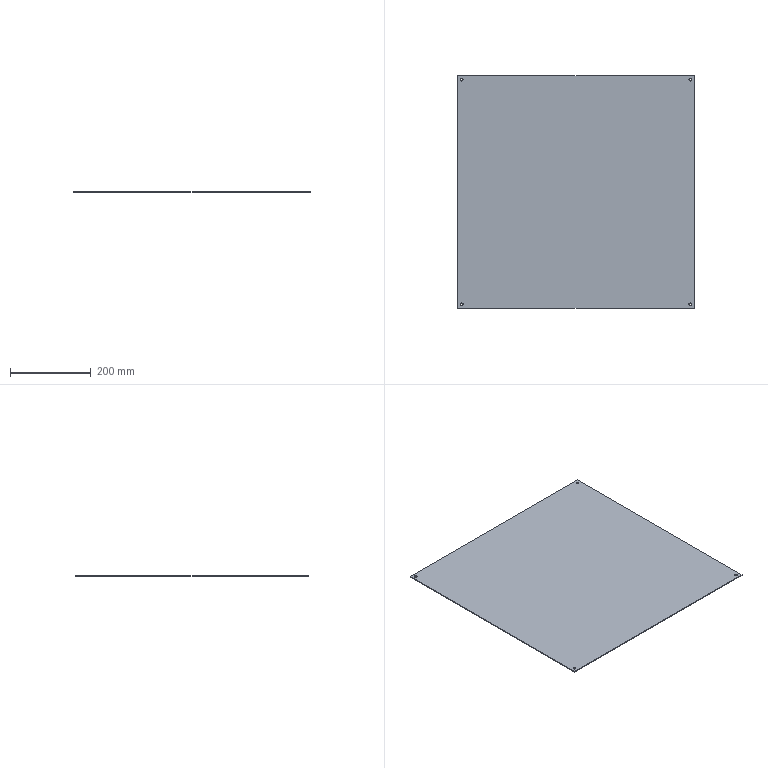Part | SolidWorks | features FlatPattern 1, HoleWzd 1, SMBaseFlange 1, SheetMetal 1 | 1 solid | 14 faces | box 587 x 577 x 2 mm | volume 677090 mm3 | cylinder 8 | plane 6 | commonest cylinder face diameters 7 x8
STEP:
#1=CARTESIAN_POINT('',(-287.,278.5,-2.));
#2=VERTEX_POINT('',#1);
#3=CARTESIAN_POINT('',(-280.,278.5,-2.));
#4=VERTEX_POINT('',#3);
#5=CARTESIAN_POINT('',(-283.5,278.5,-2.));
#6=DIRECTION('',(0.,0.,1.));
#7=DIRECTION('',(1.,0.,0.));
#8=AXIS2_PLACEMENT_3D('',#5,#6,#7);
#9=CIRCLE('',#8,3.5);
#10=EDGE_CURVE('',#2,#4,#9,.T.);
#11=ORIENTED_EDGE('',*,*,#10,.F.);
#12=CARTESIAN_POINT('',(-287.,278.5,0.));
#13=VERTEX_POINT('',#12);
#14=CARTESIAN_POINT('',(-287.,278.5,0.));
#15=DIRECTION('',(0.,0.,1.));
#16=VECTOR('',#15,1000.);
#17=LINE('',#14,#16);
#18=EDGE_CURVE('',#2,#13,#17,.T.);
#19=ORIENTED_EDGE('',*,*,#18,.T.);
#20=CARTESIAN_POINT('',(-280.,278.5,0.));
#21=VERTEX_POINT('',#20);
#22=CARTESIAN_POINT('',(-283.5,278.5,0.));
#23=DIRECTION('',(0.,0.,1.));
#24=DIRECTION('',(1.,0.,0.));
#25=AXIS2_PLACEMENT_3D('',#22,#23,#24);
#26=CIRCLE('',#25,3.5);
#27=EDGE_CURVE('',#13,#21,#26,.T.);
#28=ORIENTED_EDGE('',*,*,#27,.T.);
#29=CARTESIAN_POINT('',(-280.,278.5,0.));
#30=DIRECTION('',(0.,0.,1.));
#31=VECTOR('',#30,1000.);
#32=LINE('',#29,#31);
#33=EDGE_CURVE('',#4,#21,#32,.T.);
#34=ORIENTED_EDGE('',*,*,#33,.F.);
#35=EDGE_LOOP('',(#11,#19,#28,#34));
#36=FACE_OUTER_BOUND('',#35,.T.);
#37=CARTESIAN_POINT('',(-283.5,278.5,0.));
#38=DIRECTION('',(0.,0.,1.));
#39=DIRECTION('',(1.,0.,0.));
#40=AXIS2_PLACEMENT_3D('',#37,#38,#39);
#41=CYLINDRICAL_SURFACE('',#40,3.5);
#42=ADVANCED_FACE('',(#36),#41,.F.);
#43=CARTESIAN_POINT('',(-287.,-278.5,-2.));
#44=VERTEX_POINT('',#43);
#45=CARTESIAN_POINT('',(-280.,-278.5,-2.));
#46=VERTEX_POINT('',#45);
#47=CARTESIAN_POINT('',(-283.5,-278.5,-2.));
#48=DIRECTION('',(0.,0.,1.));
#49=DIRECTION('',(1.,0.,0.));
#50=AXIS2_PLACEMENT_3D('',#47,#48,#49);
#51=CIRCLE('',#50,3.5);
#52=EDGE_CURVE('',#44,#46,#51,.T.);
#53=ORIENTED_EDGE('',*,*,#52,.F.);
#54=CARTESIAN_POINT('',(-287.,-278.5,0.));
#55=VERTEX_POINT('',#54);
#56=CARTESIAN_POINT('',(-287.,-278.5,0.));
#57=DIRECTION('',(0.,0.,1.));
#58=VECTOR('',#57,1000.);
#59=LINE('',#56,#58);
#60=EDGE_CURVE('',#44,#55,#59,.T.);
#61=ORIENTED_EDGE('',*,*,#60,.T.);
#62=CARTESIAN_POINT('',(-280.,-278.5,0.));
#63=VERTEX_POINT('',#62);
#64=CARTESIAN_POINT('',(-283.5,-278.5,0.));
#65=DIRECTION('',(0.,0.,1.));
#66=DIRECTION('',(1.,0.,0.));
#67=AXIS2_PLACEMENT_3D('',#64,#65,#66);
#68=CIRCLE('',#67,3.5);
#69=EDGE_CURVE('',#55,#63,#68,.T.);
#70=ORIENTED_EDGE('',*,*,#69,.T.);
#71=CARTESIAN_POINT('',(-280.,-278.5,0.));
#72=DIRECTION('',(0.,0.,1.));
#73=VECTOR('',#72,1000.);
#74=LINE('',#71,#73);
#75=EDGE_CURVE('',#46,#63,#74,.T.);
#76=ORIENTED_EDGE('',*,*,#75,.F.);
#77=EDGE_LOOP('',(#53,#61,#70,#76));
#78=FACE_OUTER_BOUND('',#77,.T.);
#79=CARTESIAN_POINT('',(-283.5,-278.5,0.));
#80=DIRECTION('',(0.,0.,1.));
#81=DIRECTION('',(1.,0.,0.));
#82=AXIS2_PLACEMENT_3D('',#79,#80,#81);
#83=CYLINDRICAL_SURFACE('',#82,3.5);
#84=ADVANCED_FACE('',(#78),#83,.F.);
#85=CARTESIAN_POINT('',(280.,-278.5,-2.));
#86=VERTEX_POINT('',#85);
#87=CARTESIAN_POINT('',(287.,-278.5,-2.));
#88=VERTEX_POINT('',#87);
#89=CARTESIAN_POINT('',(283.5,-278.5,-2.));
#90=DIRECTION('',(0.,0.,1.));
#91=DIRECTION('',(1.,0.,0.));
#92=AXIS2_PLACEMENT_3D('',#89,#90,#91);
#93=CIRCLE('',#92,3.5);
#94=EDGE_CURVE('',#86,#88,#93,.T.);
#95=ORIENTED_EDGE('',*,*,#94,.F.);
#96=CARTESIAN_POINT('',(280.,-278.5,0.));
#97=VERTEX_POINT('',#96);
#98=CARTESIAN_POINT('',(280.,-278.5,0.));
#99=DIRECTION('',(0.,0.,1.));
#100=VECTOR('',#99,1000.);
#101=LINE('',#98,#100);
#102=EDGE_CURVE('',#86,#97,#101,.T.);
#103=ORIENTED_EDGE('',*,*,#102,.T.);
#104=CARTESIAN_POINT('',(287.,-278.5,0.));
#105=VERTEX_POINT('',#104);
#106=CARTESIAN_POINT('',(283.5,-278.5,0.));
#107=DIRECTION('',(0.,0.,1.));
#108=DIRECTION('',(1.,0.,0.));
#109=AXIS2_PLACEMENT_3D('',#106,#107,#108);
#110=CIRCLE('',#109,3.5);
#111=EDGE_CURVE('',#97,#105,#110,.T.);
#112=ORIENTED_EDGE('',*,*,#111,.T.);
#113=CARTESIAN_POINT('',(287.,-278.5,0.));
#114=DIRECTION('',(0.,0.,1.));
#115=VECTOR('',#114,1000.);
#116=LINE('',#113,#115);
#117=EDGE_CURVE('',#88,#105,#116,.T.);
#118=ORIENTED_EDGE('',*,*,#117,.F.);
#119=EDGE_LOOP('',(#95,#103,#112,#118));
#120=FACE_OUTER_BOUND('',#119,.T.);
#121=CARTESIAN_POINT('',(283.5,-278.5,0.));
#122=DIRECTION('',(0.,0.,1.));
#123=DIRECTION('',(1.,0.,0.));
#124=AXIS2_PLACEMENT_3D('',#121,#122,#123);
#125=CYLINDRICAL_SURFACE('',#124,3.5);
#126=ADVANCED_FACE('',(#120),#125,.F.);
#127=CARTESIAN_POINT('',(280.,278.5,-2.));
#128=VERTEX_POINT('',#127);
#129=CARTESIAN_POINT('',(287.,278.5,-2.));
#130=VERTEX_POINT('',#129);
#131=CARTESIAN_POINT('',(283.5,278.5,-2.));
#132=DIRECTION('',(0.,0.,1.));
#133=DIRECTION('',(1.,0.,0.));
#134=AXIS2_PLACEMENT_3D('',#131,#132,#133);
#135=CIRCLE('',#134,3.5);
#136=EDGE_CURVE('',#128,#130,#135,.T.);
#137=ORIENTED_EDGE('',*,*,#136,.F.);
#138=CARTESIAN_POINT('',(280.,278.5,0.));
#139=VERTEX_POINT('',#138);
#140=CARTESIAN_POINT('',(280.,278.5,0.));
#141=DIRECTION('',(0.,0.,1.));
#142=VECTOR('',#141,1000.);
#143=LINE('',#140,#142);
#144=EDGE_CURVE('',#128,#139,#143,.T.);
#145=ORIENTED_EDGE('',*,*,#144,.T.);
#146=CARTESIAN_POINT('',(287.,278.5,0.));
#147=VERTEX_POINT('',#146);
#148=CARTESIAN_POINT('',(283.5,278.5,0.));
#149=DIRECTION('',(0.,0.,1.));
#150=DIRECTION('',(1.,0.,0.));
#151=AXIS2_PLACEMENT_3D('',#148,#149,#150);
#152=CIRCLE('',#151,3.5);
#153=EDGE_CURVE('',#139,#147,#152,.T.);
#154=ORIENTED_EDGE('',*,*,#153,.T.);
#155=CARTESIAN_POINT('',(287.,278.5,0.));
#156=DIRECTION('',(0.,0.,1.));
#157=VECTOR('',#156,1000.);
#158=LINE('',#155,#157);
#159=EDGE_CURVE('',#130,#147,#158,.T.);
#160=ORIENTED_EDGE('',*,*,#159,.F.);
#161=EDGE_LOOP('',(#137,#145,#154,#160));
#162=FACE_OUTER_BOUND('',#161,.T.);
#163=CARTESIAN_POINT('',(283.5,278.5,0.));
#164=DIRECTION('',(0.,0.,1.));
#165=DIRECTION('',(1.,0.,0.));
#166=AXIS2_PLACEMENT_3D('',#163,#164,#165);
#167=CYLINDRICAL_SURFACE('',#166,3.5);
#168=ADVANCED_FACE('',(#162),#167,.F.);
#169=CARTESIAN_POINT('',(293.5,-288.5,0.));
#170=VERTEX_POINT('',#169);
#171=CARTESIAN_POINT('',(293.5,288.5,0.));
#172=VERTEX_POINT('',#171);
#173=CARTESIAN_POINT('',(293.5,288.5,0.));
#174=DIRECTION('',(0.,1.,0.));
#175=VECTOR('',#174,1000.);
#176=LINE('',#173,#175);
#177=EDGE_CURVE('',#170,#172,#176,.T.);
#178=ORIENTED_EDGE('',*,*,#177,.F.);
#179=CARTESIAN_POINT('',(293.5,-288.5,-2.));
#180=VERTEX_POINT('',#179);
#181=CARTESIAN_POINT('',(293.5,-288.5,-2.));
#182=DIRECTION('',(0.,0.,1.));
#183=VECTOR('',#182,1000.);
#184=LINE('',#181,#183);
#185=EDGE_CURVE('',#180,#170,#184,.T.);
#186=ORIENTED_EDGE('',*,*,#185,.F.);
#187=CARTESIAN_POINT('',(293.5,288.5,-2.));
#188=VERTEX_POINT('',#187);
#189=CARTESIAN_POINT('',(293.5,288.5,-2.));
#190=DIRECTION('',(0.,1.,0.));
#191=VECTOR('',#190,1000.);
#192=LINE('',#189,#191);
#193=EDGE_CURVE('',#180,#188,#192,.T.);
#194=ORIENTED_EDGE('',*,*,#193,.T.);
#195=CARTESIAN_POINT('',(293.5,288.5,-2.));
#196=DIRECTION('',(0.,0.,1.));
#197=VECTOR('',#196,1000.);
#198=LINE('',#195,#197);
#199=EDGE_CURVE('',#188,#172,#198,.T.);
#200=ORIENTED_EDGE('',*,*,#199,.T.);
#201=EDGE_LOOP('',(#178,#186,#194,#200));
#202=FACE_OUTER_BOUND('',#201,.T.);
#203=CARTESIAN_POINT('',(293.5,288.5,-2.));
#204=DIRECTION('',(1.,0.,0.));
#205=DIRECTION('',(0.,1.,0.));
#206=AXIS2_PLACEMENT_3D('',#203,#204,#205);
#207=PLANE('',#206);
#208=ADVANCED_FACE('',(#202),#207,.T.);
#209=CARTESIAN_POINT('',(-293.5,-288.5,0.));
#210=VERTEX_POINT('',#209);
#211=CARTESIAN_POINT('',(-293.5,-288.5,0.));
#212=DIRECTION('',(1.,0.,0.));
#213=VECTOR('',#212,1000.);
#214=LINE('',#211,#213);
#215=EDGE_CURVE('',#210,#170,#214,.T.);
#216=ORIENTED_EDGE('',*,*,#215,.F.);
#217=CARTESIAN_POINT('',(-293.5,-288.5,-2.));
#218=VERTEX_POINT('',#217);
#219=CARTESIAN_POINT('',(-293.5,-288.5,-2.));
#220=DIRECTION('',(0.,0.,1.));
#221=VECTOR('',#220,1000.);
#222=LINE('',#219,#221);
#223=EDGE_CURVE('',#218,#210,#222,.T.);
#224=ORIENTED_EDGE('',*,*,#223,.F.);
#225=CARTESIAN_POINT('',(-293.5,-288.5,-2.));
#226=DIRECTION('',(1.,0.,0.));
#227=VECTOR('',#226,1000.);
#228=LINE('',#225,#227);
#229=EDGE_CURVE('',#218,#180,#228,.T.);
#230=ORIENTED_EDGE('',*,*,#229,.T.);
#231=ORIENTED_EDGE('',*,*,#185,.T.);
#232=EDGE_LOOP('',(#216,#224,#230,#231));
#233=FACE_OUTER_BOUND('',#232,.T.);
#234=CARTESIAN_POINT('',(-293.5,-288.5,-2.));
#235=DIRECTION('',(0.,-1.,0.));
#236=DIRECTION('',(0.,0.,-1.));
#237=AXIS2_PLACEMENT_3D('',#234,#235,#236);
#238=PLANE('',#237);
#239=ADVANCED_FACE('',(#233),#238,.T.);
#240=CARTESIAN_POINT('',(-293.5,288.5,0.));
#241=VERTEX_POINT('',#240);
#242=CARTESIAN_POINT('',(-293.5,288.5,0.));
#243=DIRECTION('',(0.,-1.,0.));
#244=VECTOR('',#243,1000.);
#245=LINE('',#242,#244);
#246=EDGE_CURVE('',#241,#210,#245,.T.);
#247=ORIENTED_EDGE('',*,*,#246,.F.);
#248=CARTESIAN_POINT('',(-293.5,288.5,-2.));
#249=VERTEX_POINT('',#248);
#250=CARTESIAN_POINT('',(-293.5,288.5,-2.));
#251=DIRECTION('',(0.,0.,1.));
#252=VECTOR('',#251,1000.);
#253=LINE('',#250,#252);
#254=EDGE_CURVE('',#249,#241,#253,.T.);
#255=ORIENTED_EDGE('',*,*,#254,.F.);
#256=CARTESIAN_POINT('',(-293.5,288.5,-2.));
#257=DIRECTION('',(0.,-1.,0.));
#258=VECTOR('',#257,1000.);
#259=LINE('',#256,#258);
#260=EDGE_CURVE('',#249,#218,#259,.T.);
#261=ORIENTED_EDGE('',*,*,#260,.T.);
#262=ORIENTED_EDGE('',*,*,#223,.T.);
#263=EDGE_LOOP('',(#247,#255,#261,#262));
#264=FACE_OUTER_BOUND('',#263,.T.);
#265=CARTESIAN_POINT('',(-293.5,288.5,-2.));
#266=DIRECTION('',(-1.,0.,0.));
#267=DIRECTION('',(0.,-1.,0.));
#268=AXIS2_PLACEMENT_3D('',#265,#266,#267);
#269=PLANE('',#268);
#270=ADVANCED_FACE('',(#264),#269,.T.);
#271=CARTESIAN_POINT('',(-293.5,288.5,0.));
#272=DIRECTION('',(-1.,0.,0.));
#273=VECTOR('',#272,1000.);
#274=LINE('',#271,#273);
#275=EDGE_CURVE('',#172,#241,#274,.T.);
#276=ORIENTED_EDGE('',*,*,#275,.F.);
#277=ORIENTED_EDGE('',*,*,#199,.F.);
#278=CARTESIAN_POINT('',(-293.5,288.5,-2.));
#279=DIRECTION('',(-1.,0.,0.));
#280=VECTOR('',#279,1000.);
#281=LINE('',#278,#280);
#282=EDGE_CURVE('',#188,#249,#281,.T.);
#283=ORIENTED_EDGE('',*,*,#282,.T.);
#284=ORIENTED_EDGE('',*,*,#254,.T.);
#285=EDGE_LOOP('',(#276,#277,#283,#284));
#286=FACE_OUTER_BOUND('',#285,.T.);
#287=CARTESIAN_POINT('',(-293.5,288.5,-2.));
#288=DIRECTION('',(0.,1.,0.));
#289=DIRECTION('',(0.,0.,1.));
#290=AXIS2_PLACEMENT_3D('',#287,#288,#289);
#291=PLANE('',#290);
#292=ADVANCED_FACE('',(#286),#291,.T.);
#293=CARTESIAN_POINT('',(-283.5,278.5,-2.));
#294=DIRECTION('',(0.,0.,1.));
#295=DIRECTION('',(1.,0.,0.));
#296=AXIS2_PLACEMENT_3D('',#293,#294,#295);
#297=CIRCLE('',#296,3.5);
#298=EDGE_CURVE('',#4,#2,#297,.T.);
#299=ORIENTED_EDGE('',*,*,#298,.T.);
#300=ORIENTED_EDGE('',*,*,#10,.T.);
#301=EDGE_LOOP('',(#299,#300));
#302=FACE_BOUND('',#301,.T.);
#303=CARTESIAN_POINT('',(-283.5,-278.5,-2.));
#304=DIRECTION('',(0.,0.,1.));
#305=DIRECTION('',(1.,0.,0.));
#306=AXIS2_PLACEMENT_3D('',#303,#304,#305);
#307=CIRCLE('',#306,3.5);
#308=EDGE_CURVE('',#46,#44,#307,.T.);
#309=ORIENTED_EDGE('',*,*,#308,.T.);
#310=ORIENTED_EDGE('',*,*,#52,.T.);
#311=EDGE_LOOP('',(#309,#310));
#312=FACE_BOUND('',#311,.T.);
#313=CARTESIAN_POINT('',(283.5,-278.5,-2.));
#314=DIRECTION('',(0.,0.,1.));
#315=DIRECTION('',(1.,0.,0.));
#316=AXIS2_PLACEMENT_3D('',#313,#314,#315);
#317=CIRCLE('',#316,3.5);
#318=EDGE_CURVE('',#88,#86,#317,.T.);
#319=ORIENTED_EDGE('',*,*,#318,.T.);
#320=ORIENTED_EDGE('',*,*,#94,.T.);
#321=EDGE_LOOP('',(#319,#320));
#322=FACE_BOUND('',#321,.T.);
#323=CARTESIAN_POINT('',(283.5,278.5,-2.));
#324=DIRECTION('',(0.,0.,1.));
#325=DIRECTION('',(1.,0.,0.));
#326=AXIS2_PLACEMENT_3D('',#323,#324,#325);
#327=CIRCLE('',#326,3.5);
#328=EDGE_CURVE('',#130,#128,#327,.T.);
#329=ORIENTED_EDGE('',*,*,#328,.T.);
#330=ORIENTED_EDGE('',*,*,#136,.T.);
#331=EDGE_LOOP('',(#329,#330));
#332=FACE_BOUND('',#331,.T.);
#333=ORIENTED_EDGE('',*,*,#193,.F.);
#334=ORIENTED_EDGE('',*,*,#229,.F.);
#335=ORIENTED_EDGE('',*,*,#260,.F.);
#336=ORIENTED_EDGE('',*,*,#282,.F.);
#337=EDGE_LOOP('',(#333,#334,#335,#336));
#338=FACE_OUTER_BOUND('',#337,.T.);
#339=CARTESIAN_POINT('',(0.,0.,-2.));
#340=DIRECTION('',(0.,0.,1.));
#341=DIRECTION('',(1.,0.,0.));
#342=AXIS2_PLACEMENT_3D('',#339,#340,#341);
#343=PLANE('',#342);
#344=ADVANCED_FACE('',(#302,#312,#322,#332,#338),#343,.F.);
#345=CARTESIAN_POINT('',(-283.5,278.5,0.));
#346=DIRECTION('',(0.,0.,1.));
#347=DIRECTION('',(1.,0.,0.));
#348=AXIS2_PLACEMENT_3D('',#345,#346,#347);
#349=CIRCLE('',#348,3.5);
#350=EDGE_CURVE('',#21,#13,#349,.T.);
#351=ORIENTED_EDGE('',*,*,#350,.F.);
#352=ORIENTED_EDGE('',*,*,#27,.F.);
#353=EDGE_LOOP('',(#351,#352));
#354=FACE_BOUND('',#353,.T.);
#355=CARTESIAN_POINT('',(-283.5,-278.5,0.));
#356=DIRECTION('',(0.,0.,1.));
#357=DIRECTION('',(1.,0.,0.));
#358=AXIS2_PLACEMENT_3D('',#355,#356,#357);
#359=CIRCLE('',#358,3.5);
#360=EDGE_CURVE('',#63,#55,#359,.T.);
#361=ORIENTED_EDGE('',*,*,#360,.F.);
#362=ORIENTED_EDGE('',*,*,#69,.F.);
#363=EDGE_LOOP('',(#361,#362));
#364=FACE_BOUND('',#363,.T.);
#365=CARTESIAN_POINT('',(283.5,-278.5,0.));
#366=DIRECTION('',(0.,0.,1.));
#367=DIRECTION('',(1.,0.,0.));
#368=AXIS2_PLACEMENT_3D('',#365,#366,#367);
#369=CIRCLE('',#368,3.5);
#370=EDGE_CURVE('',#105,#97,#369,.T.);
#371=ORIENTED_EDGE('',*,*,#370,.F.);
#372=ORIENTED_EDGE('',*,*,#111,.F.);
#373=EDGE_LOOP('',(#371,#372));
#374=FACE_BOUND('',#373,.T.);
#375=CARTESIAN_POINT('',(283.5,278.5,0.));
#376=DIRECTION('',(0.,0.,1.));
#377=DIRECTION('',(1.,0.,0.));
#378=AXIS2_PLACEMENT_3D('',#375,#376,#377);
#379=CIRCLE('',#378,3.5);
#380=EDGE_CURVE('',#147,#139,#379,.T.);
#381=ORIENTED_EDGE('',*,*,#380,.F.);
#382=ORIENTED_EDGE('',*,*,#153,.F.);
#383=EDGE_LOOP('',(#381,#382));
#384=FACE_BOUND('',#383,.T.);
#385=ORIENTED_EDGE('',*,*,#177,.T.);
#386=ORIENTED_EDGE('',*,*,#275,.T.);
#387=ORIENTED_EDGE('',*,*,#246,.T.);
#388=ORIENTED_EDGE('',*,*,#215,.T.);
#389=EDGE_LOOP('',(#385,#386,#387,#388));
#390=FACE_OUTER_BOUND('',#389,.T.);
#391=CARTESIAN_POINT('',(0.,0.,0.));
#392=DIRECTION('',(0.,0.,1.));
#393=DIRECTION('',(1.,0.,0.));
#394=AXIS2_PLACEMENT_3D('',#391,#392,#393);
#395=PLANE('',#394);
#396=ADVANCED_FACE('',(#354,#364,#374,#384,#390),#395,.T.);
#397=ORIENTED_EDGE('',*,*,#144,.F.);
#398=ORIENTED_EDGE('',*,*,#328,.F.);
#399=ORIENTED_EDGE('',*,*,#159,.T.);
#400=ORIENTED_EDGE('',*,*,#380,.T.);
#401=EDGE_LOOP('',(#397,#398,#399,#400));
#402=FACE_OUTER_BOUND('',#401,.T.);
#403=CARTESIAN_POINT('',(283.5,278.5,0.));
#404=DIRECTION('',(0.,0.,1.));
#405=DIRECTION('',(1.,0.,0.));
#406=AXIS2_PLACEMENT_3D('',#403,#404,#405);
#407=CYLINDRICAL_SURFACE('',#406,3.5);
#408=ADVANCED_FACE('',(#402),#407,.F.);
#409=ORIENTED_EDGE('',*,*,#102,.F.);
#410=ORIENTED_EDGE('',*,*,#318,.F.);
#411=ORIENTED_EDGE('',*,*,#117,.T.);
#412=ORIENTED_EDGE('',*,*,#370,.T.);
#413=EDGE_LOOP('',(#409,#410,#411,#412));
#414=FACE_OUTER_BOUND('',#413,.T.);
#415=CARTESIAN_POINT('',(283.5,-278.5,0.));
#416=DIRECTION('',(0.,0.,1.));
#417=DIRECTION('',(1.,0.,0.));
#418=AXIS2_PLACEMENT_3D('',#415,#416,#417);
#419=CYLINDRICAL_SURFACE('',#418,3.5);
#420=ADVANCED_FACE('',(#414),#419,.F.);
#421=ORIENTED_EDGE('',*,*,#60,.F.);
#422=ORIENTED_EDGE('',*,*,#308,.F.);
#423=ORIENTED_EDGE('',*,*,#75,.T.);
#424=ORIENTED_EDGE('',*,*,#360,.T.);
#425=EDGE_LOOP('',(#421,#422,#423,#424));
#426=FACE_OUTER_BOUND('',#425,.T.);
#427=CARTESIAN_POINT('',(-283.5,-278.5,0.));
#428=DIRECTION('',(0.,0.,1.));
#429=DIRECTION('',(1.,0.,0.));
#430=AXIS2_PLACEMENT_3D('',#427,#428,#429);
#431=CYLINDRICAL_SURFACE('',#430,3.5);
#432=ADVANCED_FACE('',(#426),#431,.F.);
#433=ORIENTED_EDGE('',*,*,#18,.F.);
#434=ORIENTED_EDGE('',*,*,#298,.F.);
#435=ORIENTED_EDGE('',*,*,#33,.T.);
#436=ORIENTED_EDGE('',*,*,#350,.T.);
#437=EDGE_LOOP('',(#433,#434,#435,#436));
#438=FACE_OUTER_BOUND('',#437,.T.);
#439=CARTESIAN_POINT('',(-283.5,278.5,0.));
#440=DIRECTION('',(0.,0.,1.));
#441=DIRECTION('',(1.,0.,0.));
#442=AXIS2_PLACEMENT_3D('',#439,#440,#441);
#443=CYLINDRICAL_SURFACE('',#442,3.5);
#444=ADVANCED_FACE('',(#438),#443,.F.);
#445=CLOSED_SHELL('',(#42,#84,#126,#168,#208,#239,#270,#292,#344,#396,#408,#420,#432,#444));
#446=MANIFOLD_SOLID_BREP('',#445);
#447=CARTESIAN_POINT('',(0.,0.,0.));
#448=DIRECTION('',(0.,0.,1.));
#449=DIRECTION('',(1.,0.,0.));
#450=AXIS2_PLACEMENT_3D('',#447,#448,#449);
#451=(LENGTH_UNIT()NAMED_UNIT(*)SI_UNIT(.MILLI.,.METRE.));
#452=UNCERTAINTY_MEASURE_WITH_UNIT(LENGTH_MEASURE(0.00001),#451,'','');
#453=(NAMED_UNIT(*)PLANE_ANGLE_UNIT()SI_UNIT($,.RADIAN.));
#454=(NAMED_UNIT(*)SI_UNIT($,.STERADIAN.)SOLID_ANGLE_UNIT());
#455=(GEOMETRIC_REPRESENTATION_CONTEXT(3)GLOBAL_UNCERTAINTY_ASSIGNED_CONTEXT((#452))GLOBAL_UNIT_ASSIGNED_CONTEXT((#451,#453,#454))REPRESENTATION_CONTEXT('',''));
#456=ADVANCED_BREP_SHAPE_REPRESENTATION('',(#446,#450),#455);